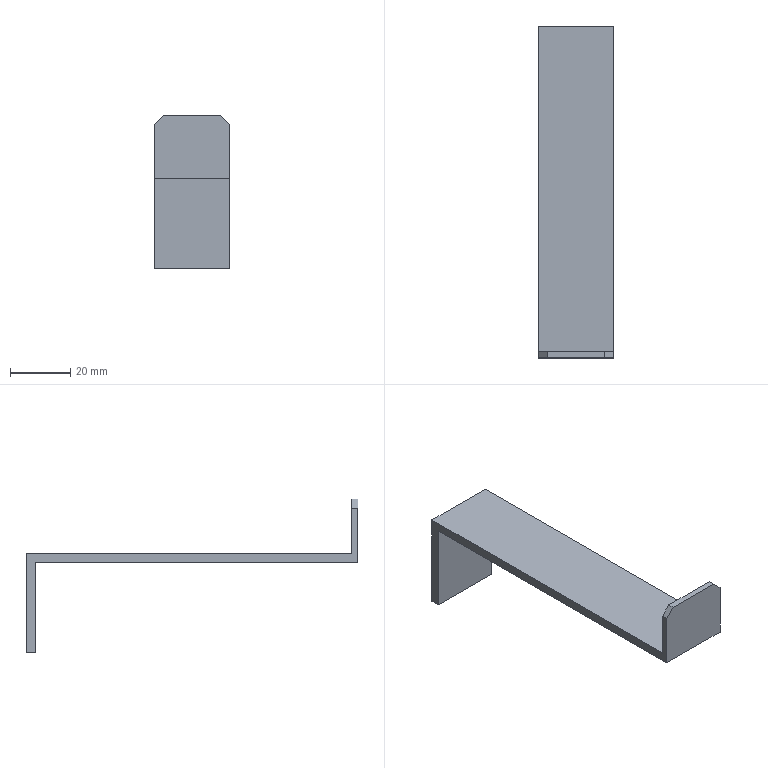Part | SolidWorks | features ICE 2, Chamfer 1, Extrusion 1 | 1 solid | 12 faces | box 25 x 110 x 51 mm | volume 11382 mm3 | plane 12
STEP:
#1=CARTESIAN_POINT('',(12.5,-53.,3.));
#2=VERTEX_POINT('',#1);
#3=CARTESIAN_POINT('',(-12.5,-53.,3.));
#4=VERTEX_POINT('',#3);
#5=CARTESIAN_POINT('',(-12.5,-53.,3.));
#6=DIRECTION('',(-1.,0.,0.));
#7=VECTOR('',#6,1000.);
#8=LINE('',#5,#7);
#9=EDGE_CURVE('',#2,#4,#8,.T.);
#10=ORIENTED_EDGE('',*,*,#9,.F.);
#11=CARTESIAN_POINT('',(12.5,55.,3.));
#12=VERTEX_POINT('',#11);
#13=CARTESIAN_POINT('',(12.5,-55.,3.));
#14=DIRECTION('',(0.,1.,0.));
#15=VECTOR('',#14,1000.);
#16=LINE('',#13,#15);
#17=EDGE_CURVE('',#2,#12,#16,.T.);
#18=ORIENTED_EDGE('',*,*,#17,.T.);
#19=CARTESIAN_POINT('',(-12.5,55.,3.));
#20=VERTEX_POINT('',#19);
#21=CARTESIAN_POINT('',(-12.5,55.,3.));
#22=DIRECTION('',(-1.,0.,0.));
#23=VECTOR('',#22,1000.);
#24=LINE('',#21,#23);
#25=EDGE_CURVE('',#12,#20,#24,.T.);
#26=ORIENTED_EDGE('',*,*,#25,.T.);
#27=CARTESIAN_POINT('',(-12.5,-55.,3.));
#28=DIRECTION('',(0.,-1.,0.));
#29=VECTOR('',#28,1000.);
#30=LINE('',#27,#29);
#31=EDGE_CURVE('',#20,#4,#30,.T.);
#32=ORIENTED_EDGE('',*,*,#31,.T.);
#33=EDGE_LOOP('',(#10,#18,#26,#32));
#34=FACE_OUTER_BOUND('',#33,.T.);
#35=CARTESIAN_POINT('',(0.,0.,3.));
#36=DIRECTION('',(0.,0.,-1.));
#37=DIRECTION('',(-1.,0.,0.));
#38=AXIS2_PLACEMENT_3D('',#35,#36,#37);
#39=PLANE('',#38);
#40=ADVANCED_FACE('',(#34),#39,.F.);
#41=CARTESIAN_POINT('',(12.5,-53.,18.));
#42=VERTEX_POINT('',#41);
#43=CARTESIAN_POINT('',(12.5,-53.,21.));
#44=DIRECTION('',(0.,0.,-1.));
#45=VECTOR('',#44,1000.);
#46=LINE('',#43,#45);
#47=EDGE_CURVE('',#42,#2,#46,.T.);
#48=ORIENTED_EDGE('',*,*,#47,.F.);
#49=CARTESIAN_POINT('',(12.5,-55.,18.));
#50=VERTEX_POINT('',#49);
#51=CARTESIAN_POINT('',(12.5,-55.,18.));
#52=DIRECTION('',(0.,-1.,0.));
#53=VECTOR('',#52,1000.);
#54=LINE('',#51,#53);
#55=EDGE_CURVE('',#42,#50,#54,.T.);
#56=ORIENTED_EDGE('',*,*,#55,.T.);
#57=CARTESIAN_POINT('',(12.5,-55.,0.));
#58=VERTEX_POINT('',#57);
#59=CARTESIAN_POINT('',(12.5,-55.,3.));
#60=DIRECTION('',(0.,0.,-1.));
#61=VECTOR('',#60,1000.);
#62=LINE('',#59,#61);
#63=EDGE_CURVE('',#50,#58,#62,.T.);
#64=ORIENTED_EDGE('',*,*,#63,.T.);
#65=CARTESIAN_POINT('',(12.5,52.,0.));
#66=VERTEX_POINT('',#65);
#67=CARTESIAN_POINT('',(12.5,-55.,0.));
#68=DIRECTION('',(0.,1.,0.));
#69=VECTOR('',#68,1000.);
#70=LINE('',#67,#69);
#71=EDGE_CURVE('',#58,#66,#70,.T.);
#72=ORIENTED_EDGE('',*,*,#71,.T.);
#73=CARTESIAN_POINT('',(12.5,52.,-30.));
#74=VERTEX_POINT('',#73);
#75=CARTESIAN_POINT('',(12.5,52.,-30.));
#76=DIRECTION('',(0.,0.,1.));
#77=VECTOR('',#76,1000.);
#78=LINE('',#75,#77);
#79=EDGE_CURVE('',#74,#66,#78,.T.);
#80=ORIENTED_EDGE('',*,*,#79,.F.);
#81=CARTESIAN_POINT('',(12.5,55.,-30.));
#82=VERTEX_POINT('',#81);
#83=CARTESIAN_POINT('',(12.5,55.,-30.));
#84=DIRECTION('',(0.,-1.,0.));
#85=VECTOR('',#84,1000.);
#86=LINE('',#83,#85);
#87=EDGE_CURVE('',#82,#74,#86,.T.);
#88=ORIENTED_EDGE('',*,*,#87,.F.);
#89=CARTESIAN_POINT('',(12.5,55.,3.));
#90=DIRECTION('',(0.,0.,-1.));
#91=VECTOR('',#90,1000.);
#92=LINE('',#89,#91);
#93=EDGE_CURVE('',#12,#82,#92,.T.);
#94=ORIENTED_EDGE('',*,*,#93,.F.);
#95=ORIENTED_EDGE('',*,*,#17,.F.);
#96=EDGE_LOOP('',(#48,#56,#64,#72,#80,#88,#94,#95));
#97=FACE_OUTER_BOUND('',#96,.T.);
#98=CARTESIAN_POINT('',(12.5,-55.,3.));
#99=DIRECTION('',(-1.,0.,0.));
#100=DIRECTION('',(0.,0.,1.));
#101=AXIS2_PLACEMENT_3D('',#98,#99,#100);
#102=PLANE('',#101);
#103=ADVANCED_FACE('',(#97),#102,.F.);
#104=ORIENTED_EDGE('',*,*,#93,.T.);
#105=CARTESIAN_POINT('',(-12.5,55.,-30.));
#106=VERTEX_POINT('',#105);
#107=CARTESIAN_POINT('',(12.5,55.,-30.));
#108=DIRECTION('',(1.,0.,0.));
#109=VECTOR('',#108,1000.);
#110=LINE('',#107,#109);
#111=EDGE_CURVE('',#106,#82,#110,.T.);
#112=ORIENTED_EDGE('',*,*,#111,.F.);
#113=CARTESIAN_POINT('',(-12.5,55.,3.));
#114=DIRECTION('',(0.,0.,-1.));
#115=VECTOR('',#114,1000.);
#116=LINE('',#113,#115);
#117=EDGE_CURVE('',#20,#106,#116,.T.);
#118=ORIENTED_EDGE('',*,*,#117,.F.);
#119=ORIENTED_EDGE('',*,*,#25,.F.);
#120=EDGE_LOOP('',(#104,#112,#118,#119));
#121=FACE_OUTER_BOUND('',#120,.T.);
#122=CARTESIAN_POINT('',(-12.5,55.,3.));
#123=DIRECTION('',(0.,-1.,0.));
#124=DIRECTION('',(0.,0.,-1.));
#125=AXIS2_PLACEMENT_3D('',#122,#123,#124);
#126=PLANE('',#125);
#127=ADVANCED_FACE('',(#121),#126,.F.);
#128=CARTESIAN_POINT('',(-12.5,-55.,18.));
#129=VERTEX_POINT('',#128);
#130=CARTESIAN_POINT('',(-12.5,-55.,0.));
#131=VERTEX_POINT('',#130);
#132=CARTESIAN_POINT('',(-12.5,-55.,3.));
#133=DIRECTION('',(0.,0.,-1.));
#134=VECTOR('',#133,1000.);
#135=LINE('',#132,#134);
#136=EDGE_CURVE('',#129,#131,#135,.T.);
#137=ORIENTED_EDGE('',*,*,#136,.F.);
#138=CARTESIAN_POINT('',(-12.5,-53.,18.));
#139=VERTEX_POINT('',#138);
#140=CARTESIAN_POINT('',(-12.5,-55.,18.));
#141=DIRECTION('',(0.,1.,0.));
#142=VECTOR('',#141,1000.);
#143=LINE('',#140,#142);
#144=EDGE_CURVE('',#129,#139,#143,.T.);
#145=ORIENTED_EDGE('',*,*,#144,.T.);
#146=CARTESIAN_POINT('',(-12.5,-53.,21.));
#147=DIRECTION('',(0.,0.,-1.));
#148=VECTOR('',#147,1000.);
#149=LINE('',#146,#148);
#150=EDGE_CURVE('',#139,#4,#149,.T.);
#151=ORIENTED_EDGE('',*,*,#150,.T.);
#152=ORIENTED_EDGE('',*,*,#31,.F.);
#153=ORIENTED_EDGE('',*,*,#117,.T.);
#154=CARTESIAN_POINT('',(-12.5,52.,-30.));
#155=VERTEX_POINT('',#154);
#156=CARTESIAN_POINT('',(-12.5,55.,-30.));
#157=DIRECTION('',(0.,1.,0.));
#158=VECTOR('',#157,1000.);
#159=LINE('',#156,#158);
#160=EDGE_CURVE('',#155,#106,#159,.T.);
#161=ORIENTED_EDGE('',*,*,#160,.F.);
#162=CARTESIAN_POINT('',(-12.5,52.,0.));
#163=VERTEX_POINT('',#162);
#164=CARTESIAN_POINT('',(-12.5,52.,-30.));
#165=DIRECTION('',(0.,0.,1.));
#166=VECTOR('',#165,1000.);
#167=LINE('',#164,#166);
#168=EDGE_CURVE('',#155,#163,#167,.T.);
#169=ORIENTED_EDGE('',*,*,#168,.T.);
#170=CARTESIAN_POINT('',(-12.5,-55.,0.));
#171=DIRECTION('',(0.,-1.,0.));
#172=VECTOR('',#171,1000.);
#173=LINE('',#170,#172);
#174=EDGE_CURVE('',#163,#131,#173,.T.);
#175=ORIENTED_EDGE('',*,*,#174,.T.);
#176=EDGE_LOOP('',(#137,#145,#151,#152,#153,#161,#169,#175));
#177=FACE_OUTER_BOUND('',#176,.T.);
#178=CARTESIAN_POINT('',(-12.5,-55.,3.));
#179=DIRECTION('',(1.,0.,0.));
#180=DIRECTION('',(0.,0.,-1.));
#181=AXIS2_PLACEMENT_3D('',#178,#179,#180);
#182=PLANE('',#181);
#183=ADVANCED_FACE('',(#177),#182,.F.);
#184=ORIENTED_EDGE('',*,*,#63,.F.);
#185=CARTESIAN_POINT('',(9.5,-55.,21.));
#186=VERTEX_POINT('',#185);
#187=CARTESIAN_POINT('',(9.5,-55.,21.));
#188=DIRECTION('',(-0.7071,0.,0.7071));
#189=VECTOR('',#188,1000.);
#190=LINE('',#187,#189);
#191=EDGE_CURVE('',#50,#186,#190,.T.);
#192=ORIENTED_EDGE('',*,*,#191,.T.);
#193=CARTESIAN_POINT('',(-9.5,-55.,21.));
#194=VERTEX_POINT('',#193);
#195=CARTESIAN_POINT('',(-12.5,-55.,21.));
#196=DIRECTION('',(1.,0.,0.));
#197=VECTOR('',#196,1000.);
#198=LINE('',#195,#197);
#199=EDGE_CURVE('',#194,#186,#198,.T.);
#200=ORIENTED_EDGE('',*,*,#199,.F.);
#201=CARTESIAN_POINT('',(-9.5,-55.,21.));
#202=DIRECTION('',(-0.7071,0.,-0.7071));
#203=VECTOR('',#202,1000.);
#204=LINE('',#201,#203);
#205=EDGE_CURVE('',#194,#129,#204,.T.);
#206=ORIENTED_EDGE('',*,*,#205,.T.);
#207=ORIENTED_EDGE('',*,*,#136,.T.);
#208=CARTESIAN_POINT('',(-12.5,-55.,0.));
#209=DIRECTION('',(1.,0.,0.));
#210=VECTOR('',#209,1000.);
#211=LINE('',#208,#210);
#212=EDGE_CURVE('',#131,#58,#211,.T.);
#213=ORIENTED_EDGE('',*,*,#212,.T.);
#214=EDGE_LOOP('',(#184,#192,#200,#206,#207,#213));
#215=FACE_OUTER_BOUND('',#214,.T.);
#216=CARTESIAN_POINT('',(-12.5,-55.,3.));
#217=DIRECTION('',(0.,1.,0.));
#218=DIRECTION('',(0.,0.,1.));
#219=AXIS2_PLACEMENT_3D('',#216,#217,#218);
#220=PLANE('',#219);
#221=ADVANCED_FACE('',(#215),#220,.F.);
#222=CARTESIAN_POINT('',(12.5,52.,0.));
#223=DIRECTION('',(-1.,0.,0.));
#224=VECTOR('',#223,1000.);
#225=LINE('',#222,#224);
#226=EDGE_CURVE('',#66,#163,#225,.T.);
#227=ORIENTED_EDGE('',*,*,#226,.F.);
#228=ORIENTED_EDGE('',*,*,#71,.F.);
#229=ORIENTED_EDGE('',*,*,#212,.F.);
#230=ORIENTED_EDGE('',*,*,#174,.F.);
#231=EDGE_LOOP('',(#227,#228,#229,#230));
#232=FACE_OUTER_BOUND('',#231,.T.);
#233=CARTESIAN_POINT('',(0.,0.,0.));
#234=DIRECTION('',(0.,0.,-1.));
#235=DIRECTION('',(-1.,0.,0.));
#236=AXIS2_PLACEMENT_3D('',#233,#234,#235);
#237=PLANE('',#236);
#238=ADVANCED_FACE('',(#232),#237,.T.);
#239=CARTESIAN_POINT('',(9.5,-53.,21.));
#240=VERTEX_POINT('',#239);
#241=CARTESIAN_POINT('',(-9.5,-53.,21.));
#242=VERTEX_POINT('',#241);
#243=CARTESIAN_POINT('',(-12.5,-53.,21.));
#244=DIRECTION('',(-1.,0.,0.));
#245=VECTOR('',#244,1000.);
#246=LINE('',#243,#245);
#247=EDGE_CURVE('',#240,#242,#246,.T.);
#248=ORIENTED_EDGE('',*,*,#247,.F.);
#249=CARTESIAN_POINT('',(9.5,-53.,21.));
#250=DIRECTION('',(0.7071,0.,-0.7071));
#251=VECTOR('',#250,1000.);
#252=LINE('',#249,#251);
#253=EDGE_CURVE('',#240,#42,#252,.T.);
#254=ORIENTED_EDGE('',*,*,#253,.T.);
#255=ORIENTED_EDGE('',*,*,#47,.T.);
#256=ORIENTED_EDGE('',*,*,#9,.T.);
#257=ORIENTED_EDGE('',*,*,#150,.F.);
#258=CARTESIAN_POINT('',(-9.5,-53.,21.));
#259=DIRECTION('',(0.7071,0.,0.7071));
#260=VECTOR('',#259,1000.);
#261=LINE('',#258,#260);
#262=EDGE_CURVE('',#139,#242,#261,.T.);
#263=ORIENTED_EDGE('',*,*,#262,.T.);
#264=EDGE_LOOP('',(#248,#254,#255,#256,#257,#263));
#265=FACE_OUTER_BOUND('',#264,.T.);
#266=CARTESIAN_POINT('',(-12.5,-53.,21.));
#267=DIRECTION('',(0.,-1.,0.));
#268=DIRECTION('',(0.,0.,-1.));
#269=AXIS2_PLACEMENT_3D('',#266,#267,#268);
#270=PLANE('',#269);
#271=ADVANCED_FACE('',(#265),#270,.F.);
#272=ORIENTED_EDGE('',*,*,#199,.T.);
#273=CARTESIAN_POINT('',(9.5,0.,21.));
#274=DIRECTION('',(0.,1.,0.));
#275=VECTOR('',#274,1000.);
#276=LINE('',#273,#275);
#277=EDGE_CURVE('',#186,#240,#276,.T.);
#278=ORIENTED_EDGE('',*,*,#277,.T.);
#279=ORIENTED_EDGE('',*,*,#247,.T.);
#280=CARTESIAN_POINT('',(-9.5,0.,21.));
#281=DIRECTION('',(0.,-1.,0.));
#282=VECTOR('',#281,1000.);
#283=LINE('',#280,#282);
#284=EDGE_CURVE('',#242,#194,#283,.T.);
#285=ORIENTED_EDGE('',*,*,#284,.T.);
#286=EDGE_LOOP('',(#272,#278,#279,#285));
#287=FACE_OUTER_BOUND('',#286,.T.);
#288=CARTESIAN_POINT('',(0.,0.,21.));
#289=DIRECTION('',(0.,0.,-1.));
#290=DIRECTION('',(-1.,0.,0.));
#291=AXIS2_PLACEMENT_3D('',#288,#289,#290);
#292=PLANE('',#291);
#293=ADVANCED_FACE('',(#287),#292,.F.);
#294=ORIENTED_EDGE('',*,*,#226,.T.);
#295=ORIENTED_EDGE('',*,*,#168,.F.);
#296=CARTESIAN_POINT('',(12.5,52.,-30.));
#297=DIRECTION('',(-1.,0.,0.));
#298=VECTOR('',#297,1000.);
#299=LINE('',#296,#298);
#300=EDGE_CURVE('',#74,#155,#299,.T.);
#301=ORIENTED_EDGE('',*,*,#300,.F.);
#302=ORIENTED_EDGE('',*,*,#79,.T.);
#303=EDGE_LOOP('',(#294,#295,#301,#302));
#304=FACE_OUTER_BOUND('',#303,.T.);
#305=CARTESIAN_POINT('',(12.5,52.,-30.));
#306=DIRECTION('',(0.,1.,0.));
#307=DIRECTION('',(0.,0.,1.));
#308=AXIS2_PLACEMENT_3D('',#305,#306,#307);
#309=PLANE('',#308);
#310=ADVANCED_FACE('',(#304),#309,.F.);
#311=ORIENTED_EDGE('',*,*,#87,.T.);
#312=ORIENTED_EDGE('',*,*,#300,.T.);
#313=ORIENTED_EDGE('',*,*,#160,.T.);
#314=ORIENTED_EDGE('',*,*,#111,.T.);
#315=EDGE_LOOP('',(#311,#312,#313,#314));
#316=FACE_OUTER_BOUND('',#315,.T.);
#317=CARTESIAN_POINT('',(0.,0.,-30.));
#318=DIRECTION('',(0.,0.,-1.));
#319=DIRECTION('',(-1.,0.,0.));
#320=AXIS2_PLACEMENT_3D('',#317,#318,#319);
#321=PLANE('',#320);
#322=ADVANCED_FACE('',(#316),#321,.T.);
#323=ORIENTED_EDGE('',*,*,#191,.F.);
#324=ORIENTED_EDGE('',*,*,#55,.F.);
#325=ORIENTED_EDGE('',*,*,#253,.F.);
#326=ORIENTED_EDGE('',*,*,#277,.F.);
#327=EDGE_LOOP('',(#323,#324,#325,#326));
#328=FACE_OUTER_BOUND('',#327,.T.);
#329=CARTESIAN_POINT('',(9.5,0.,21.));
#330=DIRECTION('',(-0.7071,0.,-0.7071));
#331=DIRECTION('',(0.,1.,0.));
#332=AXIS2_PLACEMENT_3D('',#329,#330,#331);
#333=PLANE('',#332);
#334=ADVANCED_FACE('',(#328),#333,.F.);
#335=ORIENTED_EDGE('',*,*,#262,.F.);
#336=ORIENTED_EDGE('',*,*,#144,.F.);
#337=ORIENTED_EDGE('',*,*,#205,.F.);
#338=ORIENTED_EDGE('',*,*,#284,.F.);
#339=EDGE_LOOP('',(#335,#336,#337,#338));
#340=FACE_OUTER_BOUND('',#339,.T.);
#341=CARTESIAN_POINT('',(-9.5,0.,21.));
#342=DIRECTION('',(0.7071,0.,-0.7071));
#343=DIRECTION('',(0.,-1.,0.));
#344=AXIS2_PLACEMENT_3D('',#341,#342,#343);
#345=PLANE('',#344);
#346=ADVANCED_FACE('',(#340),#345,.F.);
#347=CLOSED_SHELL('',(#40,#103,#127,#183,#221,#238,#271,#293,#310,#322,#334,#346));
#348=MANIFOLD_SOLID_BREP('',#347);
#349=CARTESIAN_POINT('',(0.,0.,0.));
#350=DIRECTION('',(0.,0.,1.));
#351=DIRECTION('',(1.,0.,0.));
#352=AXIS2_PLACEMENT_3D('',#349,#350,#351);
#353=(LENGTH_UNIT()NAMED_UNIT(*)SI_UNIT(.MILLI.,.METRE.));
#354=UNCERTAINTY_MEASURE_WITH_UNIT(LENGTH_MEASURE(0.00001),#353,'','');
#355=(NAMED_UNIT(*)PLANE_ANGLE_UNIT()SI_UNIT($,.RADIAN.));
#356=(NAMED_UNIT(*)SI_UNIT($,.STERADIAN.)SOLID_ANGLE_UNIT());
#357=(GEOMETRIC_REPRESENTATION_CONTEXT(3)GLOBAL_UNCERTAINTY_ASSIGNED_CONTEXT((#354))GLOBAL_UNIT_ASSIGNED_CONTEXT((#353,#355,#356))REPRESENTATION_CONTEXT('',''));
#358=ADVANCED_BREP_SHAPE_REPRESENTATION('',(#348,#352),#357);